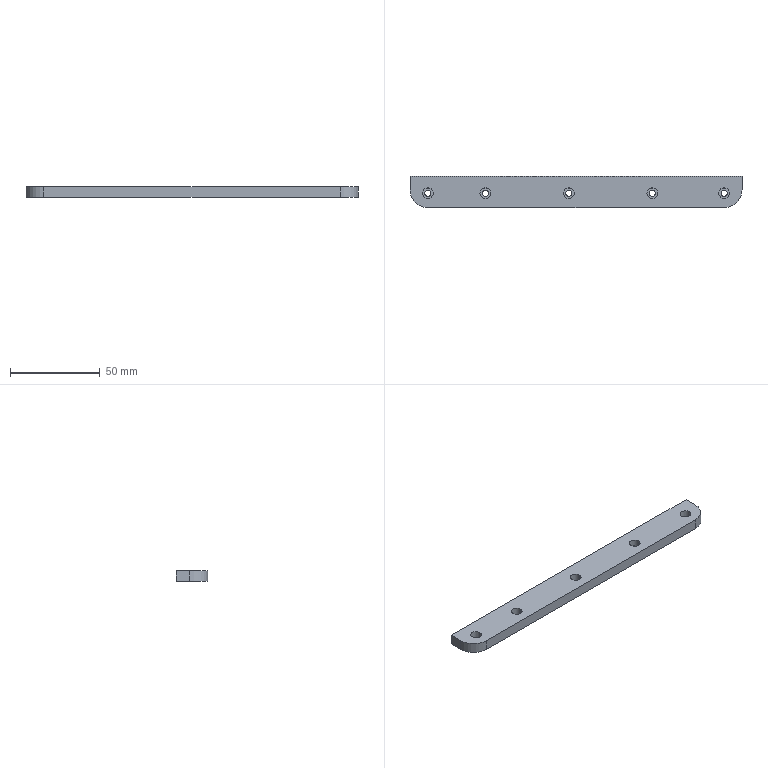Part | STEP file | PN_0009 Default | 1 solid | 33 faces | box 185 x 17.5 x 6 mm | volume 18511 mm3 | cylinder 22 | plane 11 | commonest cylinder face diameters 3.4 x10 6 x10 20 x2
STEP:
#1=CARTESIAN_POINT('',(-85.5,-0.75,2.));
#2=VERTEX_POINT('',#1);
#3=CARTESIAN_POINT('',(-79.5,-0.75,2.));
#4=VERTEX_POINT('',#3);
#5=CARTESIAN_POINT('',(-82.5,-0.75,2.));
#6=DIRECTION('',(0.,0.,1.));
#7=DIRECTION('',(1.,0.,0.));
#8=AXIS2_PLACEMENT_3D('',#5,#6,#7);
#9=CIRCLE('',#8,3.);
#10=EDGE_CURVE('',#2,#4,#9,.T.);
#11=ORIENTED_EDGE('',*,*,#10,.F.);
#12=CARTESIAN_POINT('',(-85.5,-0.75,6.));
#13=VERTEX_POINT('',#12);
#14=CARTESIAN_POINT('',(-85.5,-0.75,6.));
#15=DIRECTION('',(0.,0.,1.));
#16=VECTOR('',#15,1000.);
#17=LINE('',#14,#16);
#18=EDGE_CURVE('',#2,#13,#17,.T.);
#19=ORIENTED_EDGE('',*,*,#18,.T.);
#20=CARTESIAN_POINT('',(-79.5,-0.75,6.));
#21=VERTEX_POINT('',#20);
#22=CARTESIAN_POINT('',(-82.5,-0.75,6.));
#23=DIRECTION('',(0.,0.,1.));
#24=DIRECTION('',(1.,0.,0.));
#25=AXIS2_PLACEMENT_3D('',#22,#23,#24);
#26=CIRCLE('',#25,3.);
#27=EDGE_CURVE('',#13,#21,#26,.T.);
#28=ORIENTED_EDGE('',*,*,#27,.T.);
#29=CARTESIAN_POINT('',(-79.5,-0.75,6.));
#30=DIRECTION('',(0.,0.,1.));
#31=VECTOR('',#30,1000.);
#32=LINE('',#29,#31);
#33=EDGE_CURVE('',#4,#21,#32,.T.);
#34=ORIENTED_EDGE('',*,*,#33,.F.);
#35=EDGE_LOOP('',(#11,#19,#28,#34));
#36=FACE_OUTER_BOUND('',#35,.T.);
#37=CARTESIAN_POINT('',(-82.5,-0.75,6.));
#38=DIRECTION('',(0.,0.,1.));
#39=DIRECTION('',(1.,0.,0.));
#40=AXIS2_PLACEMENT_3D('',#37,#38,#39);
#41=CYLINDRICAL_SURFACE('',#40,3.);
#42=ADVANCED_FACE('',(#36),#41,.F.);
#43=CARTESIAN_POINT('',(-84.2,-0.75,0.));
#44=VERTEX_POINT('',#43);
#45=CARTESIAN_POINT('',(-80.8,-0.75,0.));
#46=VERTEX_POINT('',#45);
#47=CARTESIAN_POINT('',(-82.5,-0.75,0.));
#48=DIRECTION('',(0.,0.,1.));
#49=DIRECTION('',(1.,0.,0.));
#50=AXIS2_PLACEMENT_3D('',#47,#48,#49);
#51=CIRCLE('',#50,1.7);
#52=EDGE_CURVE('',#44,#46,#51,.T.);
#53=ORIENTED_EDGE('',*,*,#52,.F.);
#54=CARTESIAN_POINT('',(-84.2,-0.75,2.));
#55=VERTEX_POINT('',#54);
#56=CARTESIAN_POINT('',(-84.2,-0.75,6.));
#57=DIRECTION('',(0.,0.,1.));
#58=VECTOR('',#57,1000.);
#59=LINE('',#56,#58);
#60=EDGE_CURVE('',#44,#55,#59,.T.);
#61=ORIENTED_EDGE('',*,*,#60,.T.);
#62=CARTESIAN_POINT('',(-80.8,-0.75,2.));
#63=VERTEX_POINT('',#62);
#64=CARTESIAN_POINT('',(-82.5,-0.75,2.));
#65=DIRECTION('',(0.,0.,1.));
#66=DIRECTION('',(1.,0.,0.));
#67=AXIS2_PLACEMENT_3D('',#64,#65,#66);
#68=CIRCLE('',#67,1.7);
#69=EDGE_CURVE('',#55,#63,#68,.T.);
#70=ORIENTED_EDGE('',*,*,#69,.T.);
#71=CARTESIAN_POINT('',(-80.8,-0.75,6.));
#72=DIRECTION('',(0.,0.,1.));
#73=VECTOR('',#72,1000.);
#74=LINE('',#71,#73);
#75=EDGE_CURVE('',#46,#63,#74,.T.);
#76=ORIENTED_EDGE('',*,*,#75,.F.);
#77=EDGE_LOOP('',(#53,#61,#70,#76));
#78=FACE_OUTER_BOUND('',#77,.T.);
#79=CARTESIAN_POINT('',(-82.5,-0.75,6.));
#80=DIRECTION('',(0.,0.,1.));
#81=DIRECTION('',(1.,0.,0.));
#82=AXIS2_PLACEMENT_3D('',#79,#80,#81);
#83=CYLINDRICAL_SURFACE('',#82,1.7);
#84=ADVANCED_FACE('',(#78),#83,.F.);
#85=CARTESIAN_POINT('',(-7.,-0.75,2.));
#86=VERTEX_POINT('',#85);
#87=CARTESIAN_POINT('',(-1.,-0.75,2.));
#88=VERTEX_POINT('',#87);
#89=CARTESIAN_POINT('',(-4.,-0.75,2.));
#90=DIRECTION('',(0.,0.,1.));
#91=DIRECTION('',(1.,0.,0.));
#92=AXIS2_PLACEMENT_3D('',#89,#90,#91);
#93=CIRCLE('',#92,3.);
#94=EDGE_CURVE('',#86,#88,#93,.T.);
#95=ORIENTED_EDGE('',*,*,#94,.F.);
#96=CARTESIAN_POINT('',(-7.,-0.75,6.));
#97=VERTEX_POINT('',#96);
#98=CARTESIAN_POINT('',(-7.,-0.75,6.));
#99=DIRECTION('',(0.,0.,1.));
#100=VECTOR('',#99,1000.);
#101=LINE('',#98,#100);
#102=EDGE_CURVE('',#86,#97,#101,.T.);
#103=ORIENTED_EDGE('',*,*,#102,.T.);
#104=CARTESIAN_POINT('',(-1.,-0.75,6.));
#105=VERTEX_POINT('',#104);
#106=CARTESIAN_POINT('',(-4.,-0.75,6.));
#107=DIRECTION('',(0.,0.,1.));
#108=DIRECTION('',(1.,0.,0.));
#109=AXIS2_PLACEMENT_3D('',#106,#107,#108);
#110=CIRCLE('',#109,3.);
#111=EDGE_CURVE('',#97,#105,#110,.T.);
#112=ORIENTED_EDGE('',*,*,#111,.T.);
#113=CARTESIAN_POINT('',(-1.,-0.75,6.));
#114=DIRECTION('',(0.,0.,1.));
#115=VECTOR('',#114,1000.);
#116=LINE('',#113,#115);
#117=EDGE_CURVE('',#88,#105,#116,.T.);
#118=ORIENTED_EDGE('',*,*,#117,.F.);
#119=EDGE_LOOP('',(#95,#103,#112,#118));
#120=FACE_OUTER_BOUND('',#119,.T.);
#121=CARTESIAN_POINT('',(-4.,-0.75,6.));
#122=DIRECTION('',(0.,0.,1.));
#123=DIRECTION('',(1.,0.,0.));
#124=AXIS2_PLACEMENT_3D('',#121,#122,#123);
#125=CYLINDRICAL_SURFACE('',#124,3.);
#126=ADVANCED_FACE('',(#120),#125,.F.);
#127=CARTESIAN_POINT('',(-5.7,-0.75,0.));
#128=VERTEX_POINT('',#127);
#129=CARTESIAN_POINT('',(-2.3,-0.75,0.));
#130=VERTEX_POINT('',#129);
#131=CARTESIAN_POINT('',(-4.,-0.75,0.));
#132=DIRECTION('',(0.,0.,1.));
#133=DIRECTION('',(1.,0.,0.));
#134=AXIS2_PLACEMENT_3D('',#131,#132,#133);
#135=CIRCLE('',#134,1.7);
#136=EDGE_CURVE('',#128,#130,#135,.T.);
#137=ORIENTED_EDGE('',*,*,#136,.F.);
#138=CARTESIAN_POINT('',(-5.7,-0.75,2.));
#139=VERTEX_POINT('',#138);
#140=CARTESIAN_POINT('',(-5.7,-0.75,6.));
#141=DIRECTION('',(0.,0.,1.));
#142=VECTOR('',#141,1000.);
#143=LINE('',#140,#142);
#144=EDGE_CURVE('',#128,#139,#143,.T.);
#145=ORIENTED_EDGE('',*,*,#144,.T.);
#146=CARTESIAN_POINT('',(-2.3,-0.75,2.));
#147=VERTEX_POINT('',#146);
#148=CARTESIAN_POINT('',(-4.,-0.75,2.));
#149=DIRECTION('',(0.,0.,1.));
#150=DIRECTION('',(1.,0.,0.));
#151=AXIS2_PLACEMENT_3D('',#148,#149,#150);
#152=CIRCLE('',#151,1.7);
#153=EDGE_CURVE('',#139,#147,#152,.T.);
#154=ORIENTED_EDGE('',*,*,#153,.T.);
#155=CARTESIAN_POINT('',(-2.3,-0.75,6.));
#156=DIRECTION('',(0.,0.,1.));
#157=VECTOR('',#156,1000.);
#158=LINE('',#155,#157);
#159=EDGE_CURVE('',#130,#147,#158,.T.);
#160=ORIENTED_EDGE('',*,*,#159,.F.);
#161=EDGE_LOOP('',(#137,#145,#154,#160));
#162=FACE_OUTER_BOUND('',#161,.T.);
#163=CARTESIAN_POINT('',(-4.,-0.75,6.));
#164=DIRECTION('',(0.,0.,1.));
#165=DIRECTION('',(1.,0.,0.));
#166=AXIS2_PLACEMENT_3D('',#163,#164,#165);
#167=CYLINDRICAL_SURFACE('',#166,1.7);
#168=ADVANCED_FACE('',(#162),#167,.F.);
#169=CARTESIAN_POINT('',(39.5,-0.75,2.));
#170=VERTEX_POINT('',#169);
#171=CARTESIAN_POINT('',(45.5,-0.75,2.));
#172=VERTEX_POINT('',#171);
#173=CARTESIAN_POINT('',(42.5,-0.75,2.));
#174=DIRECTION('',(0.,0.,1.));
#175=DIRECTION('',(1.,0.,0.));
#176=AXIS2_PLACEMENT_3D('',#173,#174,#175);
#177=CIRCLE('',#176,3.);
#178=EDGE_CURVE('',#170,#172,#177,.T.);
#179=ORIENTED_EDGE('',*,*,#178,.F.);
#180=CARTESIAN_POINT('',(39.5,-0.75,6.));
#181=VERTEX_POINT('',#180);
#182=CARTESIAN_POINT('',(39.5,-0.75,6.));
#183=DIRECTION('',(0.,0.,1.));
#184=VECTOR('',#183,1000.);
#185=LINE('',#182,#184);
#186=EDGE_CURVE('',#170,#181,#185,.T.);
#187=ORIENTED_EDGE('',*,*,#186,.T.);
#188=CARTESIAN_POINT('',(45.5,-0.75,6.));
#189=VERTEX_POINT('',#188);
#190=CARTESIAN_POINT('',(42.5,-0.75,6.));
#191=DIRECTION('',(0.,0.,1.));
#192=DIRECTION('',(1.,0.,0.));
#193=AXIS2_PLACEMENT_3D('',#190,#191,#192);
#194=CIRCLE('',#193,3.);
#195=EDGE_CURVE('',#181,#189,#194,.T.);
#196=ORIENTED_EDGE('',*,*,#195,.T.);
#197=CARTESIAN_POINT('',(45.5,-0.75,6.));
#198=DIRECTION('',(0.,0.,1.));
#199=VECTOR('',#198,1000.);
#200=LINE('',#197,#199);
#201=EDGE_CURVE('',#172,#189,#200,.T.);
#202=ORIENTED_EDGE('',*,*,#201,.F.);
#203=EDGE_LOOP('',(#179,#187,#196,#202));
#204=FACE_OUTER_BOUND('',#203,.T.);
#205=CARTESIAN_POINT('',(42.5,-0.75,6.));
#206=DIRECTION('',(0.,0.,1.));
#207=DIRECTION('',(1.,0.,0.));
#208=AXIS2_PLACEMENT_3D('',#205,#206,#207);
#209=CYLINDRICAL_SURFACE('',#208,3.);
#210=ADVANCED_FACE('',(#204),#209,.F.);
#211=CARTESIAN_POINT('',(40.8,-0.75,0.));
#212=VERTEX_POINT('',#211);
#213=CARTESIAN_POINT('',(44.2,-0.75,0.));
#214=VERTEX_POINT('',#213);
#215=CARTESIAN_POINT('',(42.5,-0.75,0.));
#216=DIRECTION('',(0.,0.,1.));
#217=DIRECTION('',(1.,0.,0.));
#218=AXIS2_PLACEMENT_3D('',#215,#216,#217);
#219=CIRCLE('',#218,1.7);
#220=EDGE_CURVE('',#212,#214,#219,.T.);
#221=ORIENTED_EDGE('',*,*,#220,.F.);
#222=CARTESIAN_POINT('',(40.8,-0.75,2.));
#223=VERTEX_POINT('',#222);
#224=CARTESIAN_POINT('',(40.8,-0.75,6.));
#225=DIRECTION('',(0.,0.,1.));
#226=VECTOR('',#225,1000.);
#227=LINE('',#224,#226);
#228=EDGE_CURVE('',#212,#223,#227,.T.);
#229=ORIENTED_EDGE('',*,*,#228,.T.);
#230=CARTESIAN_POINT('',(44.2,-0.75,2.));
#231=VERTEX_POINT('',#230);
#232=CARTESIAN_POINT('',(42.5,-0.75,2.));
#233=DIRECTION('',(0.,0.,1.));
#234=DIRECTION('',(1.,0.,0.));
#235=AXIS2_PLACEMENT_3D('',#232,#233,#234);
#236=CIRCLE('',#235,1.7);
#237=EDGE_CURVE('',#223,#231,#236,.T.);
#238=ORIENTED_EDGE('',*,*,#237,.T.);
#239=CARTESIAN_POINT('',(44.2,-0.75,6.));
#240=DIRECTION('',(0.,0.,1.));
#241=VECTOR('',#240,1000.);
#242=LINE('',#239,#241);
#243=EDGE_CURVE('',#214,#231,#242,.T.);
#244=ORIENTED_EDGE('',*,*,#243,.F.);
#245=EDGE_LOOP('',(#221,#229,#238,#244));
#246=FACE_OUTER_BOUND('',#245,.T.);
#247=CARTESIAN_POINT('',(42.5,-0.75,6.));
#248=DIRECTION('',(0.,0.,1.));
#249=DIRECTION('',(1.,0.,0.));
#250=AXIS2_PLACEMENT_3D('',#247,#248,#249);
#251=CYLINDRICAL_SURFACE('',#250,1.7);
#252=ADVANCED_FACE('',(#246),#251,.F.);
#253=CARTESIAN_POINT('',(-53.5,-0.75,2.));
#254=VERTEX_POINT('',#253);
#255=CARTESIAN_POINT('',(-47.5,-0.75,2.));
#256=VERTEX_POINT('',#255);
#257=CARTESIAN_POINT('',(-50.5,-0.75,2.));
#258=DIRECTION('',(0.,0.,1.));
#259=DIRECTION('',(1.,0.,0.));
#260=AXIS2_PLACEMENT_3D('',#257,#258,#259);
#261=CIRCLE('',#260,3.);
#262=EDGE_CURVE('',#254,#256,#261,.T.);
#263=ORIENTED_EDGE('',*,*,#262,.F.);
#264=CARTESIAN_POINT('',(-53.5,-0.75,6.));
#265=VERTEX_POINT('',#264);
#266=CARTESIAN_POINT('',(-53.5,-0.75,6.));
#267=DIRECTION('',(0.,0.,1.));
#268=VECTOR('',#267,1000.);
#269=LINE('',#266,#268);
#270=EDGE_CURVE('',#254,#265,#269,.T.);
#271=ORIENTED_EDGE('',*,*,#270,.T.);
#272=CARTESIAN_POINT('',(-47.5,-0.75,6.));
#273=VERTEX_POINT('',#272);
#274=CARTESIAN_POINT('',(-50.5,-0.75,6.));
#275=DIRECTION('',(0.,0.,1.));
#276=DIRECTION('',(1.,0.,0.));
#277=AXIS2_PLACEMENT_3D('',#274,#275,#276);
#278=CIRCLE('',#277,3.);
#279=EDGE_CURVE('',#265,#273,#278,.T.);
#280=ORIENTED_EDGE('',*,*,#279,.T.);
#281=CARTESIAN_POINT('',(-47.5,-0.75,6.));
#282=DIRECTION('',(0.,0.,1.));
#283=VECTOR('',#282,1000.);
#284=LINE('',#281,#283);
#285=EDGE_CURVE('',#256,#273,#284,.T.);
#286=ORIENTED_EDGE('',*,*,#285,.F.);
#287=EDGE_LOOP('',(#263,#271,#280,#286));
#288=FACE_OUTER_BOUND('',#287,.T.);
#289=CARTESIAN_POINT('',(-50.5,-0.75,6.));
#290=DIRECTION('',(0.,0.,1.));
#291=DIRECTION('',(1.,0.,0.));
#292=AXIS2_PLACEMENT_3D('',#289,#290,#291);
#293=CYLINDRICAL_SURFACE('',#292,3.);
#294=ADVANCED_FACE('',(#288),#293,.F.);
#295=CARTESIAN_POINT('',(-52.2,-0.75,0.));
#296=VERTEX_POINT('',#295);
#297=CARTESIAN_POINT('',(-48.8,-0.75,0.));
#298=VERTEX_POINT('',#297);
#299=CARTESIAN_POINT('',(-50.5,-0.75,0.));
#300=DIRECTION('',(0.,0.,1.));
#301=DIRECTION('',(1.,0.,0.));
#302=AXIS2_PLACEMENT_3D('',#299,#300,#301);
#303=CIRCLE('',#302,1.7);
#304=EDGE_CURVE('',#296,#298,#303,.T.);
#305=ORIENTED_EDGE('',*,*,#304,.F.);
#306=CARTESIAN_POINT('',(-52.2,-0.75,2.));
#307=VERTEX_POINT('',#306);
#308=CARTESIAN_POINT('',(-52.2,-0.75,6.));
#309=DIRECTION('',(0.,0.,1.));
#310=VECTOR('',#309,1000.);
#311=LINE('',#308,#310);
#312=EDGE_CURVE('',#296,#307,#311,.T.);
#313=ORIENTED_EDGE('',*,*,#312,.T.);
#314=CARTESIAN_POINT('',(-48.8,-0.75,2.));
#315=VERTEX_POINT('',#314);
#316=CARTESIAN_POINT('',(-50.5,-0.75,2.));
#317=DIRECTION('',(0.,0.,1.));
#318=DIRECTION('',(1.,0.,0.));
#319=AXIS2_PLACEMENT_3D('',#316,#317,#318);
#320=CIRCLE('',#319,1.7);
#321=EDGE_CURVE('',#307,#315,#320,.T.);
#322=ORIENTED_EDGE('',*,*,#321,.T.);
#323=CARTESIAN_POINT('',(-48.8,-0.75,6.));
#324=DIRECTION('',(0.,0.,1.));
#325=VECTOR('',#324,1000.);
#326=LINE('',#323,#325);
#327=EDGE_CURVE('',#298,#315,#326,.T.);
#328=ORIENTED_EDGE('',*,*,#327,.F.);
#329=EDGE_LOOP('',(#305,#313,#322,#328));
#330=FACE_OUTER_BOUND('',#329,.T.);
#331=CARTESIAN_POINT('',(-50.5,-0.75,6.));
#332=DIRECTION('',(0.,0.,1.));
#333=DIRECTION('',(1.,0.,0.));
#334=AXIS2_PLACEMENT_3D('',#331,#332,#333);
#335=CYLINDRICAL_SURFACE('',#334,1.7);
#336=ADVANCED_FACE('',(#330),#335,.F.);
#337=CARTESIAN_POINT('',(79.5,-0.75,2.));
#338=VERTEX_POINT('',#337);
#339=CARTESIAN_POINT('',(85.5,-0.75,2.));
#340=VERTEX_POINT('',#339);
#341=CARTESIAN_POINT('',(82.5,-0.75,2.));
#342=DIRECTION('',(0.,0.,1.));
#343=DIRECTION('',(1.,0.,0.));
#344=AXIS2_PLACEMENT_3D('',#341,#342,#343);
#345=CIRCLE('',#344,3.);
#346=EDGE_CURVE('',#338,#340,#345,.T.);
#347=ORIENTED_EDGE('',*,*,#346,.F.);
#348=CARTESIAN_POINT('',(79.5,-0.75,6.));
#349=VERTEX_POINT('',#348);
#350=CARTESIAN_POINT('',(79.5,-0.75,6.));
#351=DIRECTION('',(0.,0.,1.));
#352=VECTOR('',#351,1000.);
#353=LINE('',#350,#352);
#354=EDGE_CURVE('',#338,#349,#353,.T.);
#355=ORIENTED_EDGE('',*,*,#354,.T.);
#356=CARTESIAN_POINT('',(85.5,-0.75,6.));
#357=VERTEX_POINT('',#356);
#358=CARTESIAN_POINT('',(82.5,-0.75,6.));
#359=DIRECTION('',(0.,0.,1.));
#360=DIRECTION('',(1.,0.,0.));
#361=AXIS2_PLACEMENT_3D('',#358,#359,#360);
#362=CIRCLE('',#361,3.);
#363=EDGE_CURVE('',#349,#357,#362,.T.);
#364=ORIENTED_EDGE('',*,*,#363,.T.);
#365=CARTESIAN_POINT('',(85.5,-0.75,6.));
#366=DIRECTION('',(0.,0.,1.));
#367=VECTOR('',#366,1000.);
#368=LINE('',#365,#367);
#369=EDGE_CURVE('',#340,#357,#368,.T.);
#370=ORIENTED_EDGE('',*,*,#369,.F.);
#371=EDGE_LOOP('',(#347,#355,#364,#370));
#372=FACE_OUTER_BOUND('',#371,.T.);
#373=CARTESIAN_POINT('',(82.5,-0.75,6.));
#374=DIRECTION('',(0.,0.,1.));
#375=DIRECTION('',(1.,0.,0.));
#376=AXIS2_PLACEMENT_3D('',#373,#374,#375);
#377=CYLINDRICAL_SURFACE('',#376,3.);
#378=ADVANCED_FACE('',(#372),#377,.F.);
#379=CARTESIAN_POINT('',(80.8,-0.75,0.));
#380=VERTEX_POINT('',#379);
#381=CARTESIAN_POINT('',(84.2,-0.75,0.));
#382=VERTEX_POINT('',#381);
#383=CARTESIAN_POINT('',(82.5,-0.75,0.));
#384=DIRECTION('',(0.,0.,1.));
#385=DIRECTION('',(1.,0.,0.));
#386=AXIS2_PLACEMENT_3D('',#383,#384,#385);
#387=CIRCLE('',#386,1.7);
#388=EDGE_CURVE('',#380,#382,#387,.T.);
#389=ORIENTED_EDGE('',*,*,#388,.F.);
#390=CARTESIAN_POINT('',(80.8,-0.75,2.));
#391=VERTEX_POINT('',#390);
#392=CARTESIAN_POINT('',(80.8,-0.75,6.));
#393=DIRECTION('',(0.,0.,1.));
#394=VECTOR('',#393,1000.);
#395=LINE('',#392,#394);
#396=EDGE_CURVE('',#380,#391,#395,.T.);
#397=ORIENTED_EDGE('',*,*,#396,.T.);
#398=CARTESIAN_POINT('',(84.2,-0.75,2.));
#399=VERTEX_POINT('',#398);
#400=CARTESIAN_POINT('',(82.5,-0.75,2.));
#401=DIRECTION('',(0.,0.,1.));
#402=DIRECTION('',(1.,0.,0.));
#403=AXIS2_PLACEMENT_3D('',#400,#401,#402);
#404=CIRCLE('',#403,1.7);
#405=EDGE_CURVE('',#391,#399,#404,.T.);
#406=ORIENTED_EDGE('',*,*,#405,.T.);
#407=CARTESIAN_POINT('',(84.2,-0.75,6.));
#408=DIRECTION('',(0.,0.,1.));
#409=VECTOR('',#408,1000.);
#410=LINE('',#407,#409);
#411=EDGE_CURVE('',#382,#399,#410,.T.);
#412=ORIENTED_EDGE('',*,*,#411,.F.);
#413=EDGE_LOOP('',(#389,#397,#406,#412));
#414=FACE_OUTER_BOUND('',#413,.T.);
#415=CARTESIAN_POINT('',(82.5,-0.75,6.));
#416=DIRECTION('',(0.,0.,1.));
#417=DIRECTION('',(1.,0.,0.));
#418=AXIS2_PLACEMENT_3D('',#415,#416,#417);
#419=CYLINDRICAL_SURFACE('',#418,1.7);
#420=ADVANCED_FACE('',(#414),#419,.F.);
#421=CARTESIAN_POINT('',(92.5,1.25,6.));
#422=VERTEX_POINT('',#421);
#423=CARTESIAN_POINT('',(92.5,8.75,6.));
#424=VERTEX_POINT('',#423);
#425=CARTESIAN_POINT('',(92.5,8.75,6.));
#426=DIRECTION('',(0.,1.,0.));
#427=VECTOR('',#426,1000.);
#428=LINE('',#425,#427);
#429=EDGE_CURVE('',#422,#424,#428,.T.);
#430=ORIENTED_EDGE('',*,*,#429,.F.);
#431=CARTESIAN_POINT('',(92.5,1.25,0.));
#432=VERTEX_POINT('',#431);
#433=CARTESIAN_POINT('',(92.5,1.25,6.));
#434=DIRECTION('',(0.,0.,-1.));
#435=VECTOR('',#434,1000.);
#436=LINE('',#433,#435);
#437=EDGE_CURVE('',#422,#432,#436,.T.);
#438=ORIENTED_EDGE('',*,*,#437,.T.);
#439=CARTESIAN_POINT('',(92.5,8.75,0.));
#440=VERTEX_POINT('',#439);
#441=CARTESIAN_POINT('',(92.5,8.75,0.));
#442=DIRECTION('',(0.,1.,0.));
#443=VECTOR('',#442,1000.);
#444=LINE('',#441,#443);
#445=EDGE_CURVE('',#432,#440,#444,.T.);
#446=ORIENTED_EDGE('',*,*,#445,.T.);
#447=CARTESIAN_POINT('',(92.5,8.75,6.));
#448=DIRECTION('',(0.,0.,-1.));
#449=VECTOR('',#448,1000.);
#450=LINE('',#447,#449);
#451=EDGE_CURVE('',#424,#440,#450,.T.);
#452=ORIENTED_EDGE('',*,*,#451,.F.);
#453=EDGE_LOOP('',(#430,#438,#446,#452));
#454=FACE_OUTER_BOUND('',#453,.T.);
#455=CARTESIAN_POINT('',(92.5,8.75,6.));
#456=DIRECTION('',(-1.,0.,0.));
#457=DIRECTION('',(0.,0.,1.));
#458=AXIS2_PLACEMENT_3D('',#455,#456,#457);
#459=PLANE('',#458);
#460=ADVANCED_FACE('',(#454),#459,.F.);
#461=CARTESIAN_POINT('',(-92.5,8.75,0.));
#462=VERTEX_POINT('',#461);
#463=CARTESIAN_POINT('',(-92.5,8.75,0.));
#464=DIRECTION('',(-1.,0.,0.));
#465=VECTOR('',#464,1000.);
#466=LINE('',#463,#465);
#467=EDGE_CURVE('',#440,#462,#466,.T.);
#468=ORIENTED_EDGE('',*,*,#467,.T.);
#469=CARTESIAN_POINT('',(-92.5,8.75,6.));
#470=VERTEX_POINT('',#469);
#471=CARTESIAN_POINT('',(-92.5,8.75,6.));
#472=DIRECTION('',(0.,0.,-1.));
#473=VECTOR('',#472,1000.);
#474=LINE('',#471,#473);
#475=EDGE_CURVE('',#470,#462,#474,.T.);
#476=ORIENTED_EDGE('',*,*,#475,.F.);
#477=CARTESIAN_POINT('',(-92.5,8.75,6.));
#478=DIRECTION('',(-1.,0.,0.));
#479=VECTOR('',#478,1000.);
#480=LINE('',#477,#479);
#481=EDGE_CURVE('',#424,#470,#480,.T.);
#482=ORIENTED_EDGE('',*,*,#481,.F.);
#483=ORIENTED_EDGE('',*,*,#451,.T.);
#484=EDGE_LOOP('',(#468,#476,#482,#483));
#485=FACE_OUTER_BOUND('',#484,.T.);
#486=CARTESIAN_POINT('',(-92.5,8.75,6.));
#487=DIRECTION('',(0.,-1.,0.));
#488=DIRECTION('',(0.,0.,-1.));
#489=AXIS2_PLACEMENT_3D('',#486,#487,#488);
#490=PLANE('',#489);
#491=ADVANCED_FACE('',(#485),#490,.F.);
#492=CARTESIAN_POINT('',(-92.5,1.25,0.));
#493=VERTEX_POINT('',#492);
#494=CARTESIAN_POINT('',(-92.5,8.75,0.));
#495=DIRECTION('',(0.,-1.,0.));
#496=VECTOR('',#495,1000.);
#497=LINE('',#494,#496);
#498=EDGE_CURVE('',#462,#493,#497,.T.);
#499=ORIENTED_EDGE('',*,*,#498,.T.);
#500=CARTESIAN_POINT('',(-92.5,1.25,6.));
#501=VERTEX_POINT('',#500);
#502=CARTESIAN_POINT('',(-92.5,1.25,6.));
#503=DIRECTION('',(0.,0.,1.));
#504=VECTOR('',#503,1000.);
#505=LINE('',#502,#504);
#506=EDGE_CURVE('',#493,#501,#505,.T.);
#507=ORIENTED_EDGE('',*,*,#506,.T.);
#508=CARTESIAN_POINT('',(-92.5,8.75,6.));
#509=DIRECTION('',(0.,-1.,0.));
#510=VECTOR('',#509,1000.);
#511=LINE('',#508,#510);
#512=EDGE_CURVE('',#470,#501,#511,.T.);
#513=ORIENTED_EDGE('',*,*,#512,.F.);
#514=ORIENTED_EDGE('',*,*,#475,.T.);
#515=EDGE_LOOP('',(#499,#507,#513,#514));
#516=FACE_OUTER_BOUND('',#515,.T.);
#517=CARTESIAN_POINT('',(-92.5,8.75,6.));
#518=DIRECTION('',(1.,0.,0.));
#519=DIRECTION('',(0.,0.,-1.));
#520=AXIS2_PLACEMENT_3D('',#517,#518,#519);
#521=PLANE('',#520);
#522=ADVANCED_FACE('',(#516),#521,.F.);
#523=CARTESIAN_POINT('',(-82.5,-8.75,0.));
#524=VERTEX_POINT('',#523);
#525=CARTESIAN_POINT('',(82.5,-8.75,0.));
#526=VERTEX_POINT('',#525);
#527=CARTESIAN_POINT('',(-92.5,-8.75,0.));
#528=DIRECTION('',(1.,0.,0.));
#529=VECTOR('',#528,1000.);
#530=LINE('',#527,#529);
#531=EDGE_CURVE('',#524,#526,#530,.T.);
#532=ORIENTED_EDGE('',*,*,#531,.T.);
#533=CARTESIAN_POINT('',(82.5,-8.75,6.));
#534=VERTEX_POINT('',#533);
#535=CARTESIAN_POINT('',(82.5,-8.75,6.));
#536=DIRECTION('',(0.,0.,1.));
#537=VECTOR('',#536,1000.);
#538=LINE('',#535,#537);
#539=EDGE_CURVE('',#526,#534,#538,.T.);
#540=ORIENTED_EDGE('',*,*,#539,.T.);
#541=CARTESIAN_POINT('',(-82.5,-8.75,6.));
#542=VERTEX_POINT('',#541);
#543=CARTESIAN_POINT('',(-92.5,-8.75,6.));
#544=DIRECTION('',(1.,0.,0.));
#545=VECTOR('',#544,1000.);
#546=LINE('',#543,#545);
#547=EDGE_CURVE('',#542,#534,#546,.T.);
#548=ORIENTED_EDGE('',*,*,#547,.F.);
#549=CARTESIAN_POINT('',(-82.5,-8.75,6.));
#550=DIRECTION('',(0.,0.,-1.));
#551=VECTOR('',#550,1000.);
#552=LINE('',#549,#551);
#553=EDGE_CURVE('',#542,#524,#552,.T.);
#554=ORIENTED_EDGE('',*,*,#553,.T.);
#555=EDGE_LOOP('',(#532,#540,#548,#554));
#556=FACE_OUTER_BOUND('',#555,.T.);
#557=CARTESIAN_POINT('',(-92.5,-8.75,6.));
#558=DIRECTION('',(0.,1.,0.));
#559=DIRECTION('',(0.,0.,1.));
#560=AXIS2_PLACEMENT_3D('',#557,#558,#559);
#561=PLANE('',#560);
#562=ADVANCED_FACE('',(#556),#561,.F.);
#563=CARTESIAN_POINT('',(-82.5,-0.75,6.));
#564=DIRECTION('',(0.,0.,1.));
#565=DIRECTION('',(1.,0.,0.));
#566=AXIS2_PLACEMENT_3D('',#563,#564,#565);
#567=CIRCLE('',#566,3.);
#568=EDGE_CURVE('',#21,#13,#567,.T.);
#569=ORIENTED_EDGE('',*,*,#568,.F.);
#570=ORIENTED_EDGE('',*,*,#27,.F.);
#571=EDGE_LOOP('',(#569,#570));
#572=FACE_BOUND('',#571,.T.);
#573=CARTESIAN_POINT('',(-4.,-0.75,6.));
#574=DIRECTION('',(0.,0.,1.));
#575=DIRECTION('',(1.,0.,0.));
#576=AXIS2_PLACEMENT_3D('',#573,#574,#575);
#577=CIRCLE('',#576,3.);
#578=EDGE_CURVE('',#105,#97,#577,.T.);
#579=ORIENTED_EDGE('',*,*,#578,.F.);
#580=ORIENTED_EDGE('',*,*,#111,.F.);
#581=EDGE_LOOP('',(#579,#580));
#582=FACE_BOUND('',#581,.T.);
#583=CARTESIAN_POINT('',(42.5,-0.75,6.));
#584=DIRECTION('',(0.,0.,1.));
#585=DIRECTION('',(1.,0.,0.));
#586=AXIS2_PLACEMENT_3D('',#583,#584,#585);
#587=CIRCLE('',#586,3.);
#588=EDGE_CURVE('',#189,#181,#587,.T.);
#589=ORIENTED_EDGE('',*,*,#588,.F.);
#590=ORIENTED_EDGE('',*,*,#195,.F.);
#591=EDGE_LOOP('',(#589,#590));
#592=FACE_BOUND('',#591,.T.);
#593=CARTESIAN_POINT('',(-50.5,-0.75,6.));
#594=DIRECTION('',(0.,0.,1.));
#595=DIRECTION('',(1.,0.,0.));
#596=AXIS2_PLACEMENT_3D('',#593,#594,#595);
#597=CIRCLE('',#596,3.);
#598=EDGE_CURVE('',#273,#265,#597,.T.);
#599=ORIENTED_EDGE('',*,*,#598,.F.);
#600=ORIENTED_EDGE('',*,*,#279,.F.);
#601=EDGE_LOOP('',(#599,#600));
#602=FACE_BOUND('',#601,.T.);
#603=CARTESIAN_POINT('',(82.5,-0.75,6.));
#604=DIRECTION('',(0.,0.,1.));
#605=DIRECTION('',(1.,0.,0.));
#606=AXIS2_PLACEMENT_3D('',#603,#604,#605);
#607=CIRCLE('',#606,3.);
#608=EDGE_CURVE('',#357,#349,#607,.T.);
#609=ORIENTED_EDGE('',*,*,#608,.F.);
#610=ORIENTED_EDGE('',*,*,#363,.F.);
#611=EDGE_LOOP('',(#609,#610));
#612=FACE_BOUND('',#611,.T.);
#613=ORIENTED_EDGE('',*,*,#547,.T.);
#614=CARTESIAN_POINT('',(82.5,1.25,6.));
#615=DIRECTION('',(0.,0.,1.));
#616=DIRECTION('',(1.,0.,0.));
#617=AXIS2_PLACEMENT_3D('',#614,#615,#616);
#618=CIRCLE('',#617,10.);
#619=EDGE_CURVE('',#534,#422,#618,.T.);
#620=ORIENTED_EDGE('',*,*,#619,.T.);
#621=ORIENTED_EDGE('',*,*,#429,.T.);
#622=ORIENTED_EDGE('',*,*,#481,.T.);
#623=ORIENTED_EDGE('',*,*,#512,.T.);
#624=CARTESIAN_POINT('',(-82.5,1.25,6.));
#625=DIRECTION('',(0.,0.,1.));
#626=DIRECTION('',(1.,0.,0.));
#627=AXIS2_PLACEMENT_3D('',#624,#625,#626);
#628=CIRCLE('',#627,10.);
#629=EDGE_CURVE('',#501,#542,#628,.T.);
#630=ORIENTED_EDGE('',*,*,#629,.T.);
#631=EDGE_LOOP('',(#613,#620,#621,#622,#623,#630));
#632=FACE_OUTER_BOUND('',#631,.T.);
#633=CARTESIAN_POINT('',(0.,0.,6.));
#634=DIRECTION('',(0.,0.,1.));
#635=DIRECTION('',(1.,0.,0.));
#636=AXIS2_PLACEMENT_3D('',#633,#634,#635);
#637=PLANE('',#636);
#638=ADVANCED_FACE('',(#572,#582,#592,#602,#612,#632),#637,.T.);
#639=CARTESIAN_POINT('',(-82.5,-0.75,0.));
#640=DIRECTION('',(0.,0.,1.));
#641=DIRECTION('',(1.,0.,0.));
#642=AXIS2_PLACEMENT_3D('',#639,#640,#641);
#643=CIRCLE('',#642,1.7);
#644=EDGE_CURVE('',#46,#44,#643,.T.);
#645=ORIENTED_EDGE('',*,*,#644,.T.);
#646=ORIENTED_EDGE('',*,*,#52,.T.);
#647=EDGE_LOOP('',(#645,#646));
#648=FACE_BOUND('',#647,.T.);
#649=CARTESIAN_POINT('',(-4.,-0.75,0.));
#650=DIRECTION('',(0.,0.,1.));
#651=DIRECTION('',(1.,0.,0.));
#652=AXIS2_PLACEMENT_3D('',#649,#650,#651);
#653=CIRCLE('',#652,1.7);
#654=EDGE_CURVE('',#130,#128,#653,.T.);
#655=ORIENTED_EDGE('',*,*,#654,.T.);
#656=ORIENTED_EDGE('',*,*,#136,.T.);
#657=EDGE_LOOP('',(#655,#656));
#658=FACE_BOUND('',#657,.T.);
#659=CARTESIAN_POINT('',(42.5,-0.75,0.));
#660=DIRECTION('',(0.,0.,1.));
#661=DIRECTION('',(1.,0.,0.));
#662=AXIS2_PLACEMENT_3D('',#659,#660,#661);
#663=CIRCLE('',#662,1.7);
#664=EDGE_CURVE('',#214,#212,#663,.T.);
#665=ORIENTED_EDGE('',*,*,#664,.T.);
#666=ORIENTED_EDGE('',*,*,#220,.T.);
#667=EDGE_LOOP('',(#665,#666));
#668=FACE_BOUND('',#667,.T.);
#669=CARTESIAN_POINT('',(-50.5,-0.75,0.));
#670=DIRECTION('',(0.,0.,1.));
#671=DIRECTION('',(1.,0.,0.));
#672=AXIS2_PLACEMENT_3D('',#669,#670,#671);
#673=CIRCLE('',#672,1.7);
#674=EDGE_CURVE('',#298,#296,#673,.T.);
#675=ORIENTED_EDGE('',*,*,#674,.T.);
#676=ORIENTED_EDGE('',*,*,#304,.T.);
#677=EDGE_LOOP('',(#675,#676));
#678=FACE_BOUND('',#677,.T.);
#679=CARTESIAN_POINT('',(82.5,-0.75,0.));
#680=DIRECTION('',(0.,0.,1.));
#681=DIRECTION('',(1.,0.,0.));
#682=AXIS2_PLACEMENT_3D('',#679,#680,#681);
#683=CIRCLE('',#682,1.7);
#684=EDGE_CURVE('',#382,#380,#683,.T.);
#685=ORIENTED_EDGE('',*,*,#684,.T.);
#686=ORIENTED_EDGE('',*,*,#388,.T.);
#687=EDGE_LOOP('',(#685,#686));
#688=FACE_BOUND('',#687,.T.);
#689=ORIENTED_EDGE('',*,*,#445,.F.);
#690=CARTESIAN_POINT('',(82.5,1.25,0.));
#691=DIRECTION('',(0.,0.,-1.));
#692=DIRECTION('',(1.,0.,0.));
#693=AXIS2_PLACEMENT_3D('',#690,#691,#692);
#694=CIRCLE('',#693,10.);
#695=EDGE_CURVE('',#432,#526,#694,.T.);
#696=ORIENTED_EDGE('',*,*,#695,.T.);
#697=ORIENTED_EDGE('',*,*,#531,.F.);
#698=CARTESIAN_POINT('',(-82.5,1.25,0.));
#699=DIRECTION('',(0.,0.,-1.));
#700=DIRECTION('',(1.,0.,0.));
#701=AXIS2_PLACEMENT_3D('',#698,#699,#700);
#702=CIRCLE('',#701,10.);
#703=EDGE_CURVE('',#524,#493,#702,.T.);
#704=ORIENTED_EDGE('',*,*,#703,.T.);
#705=ORIENTED_EDGE('',*,*,#498,.F.);
#706=ORIENTED_EDGE('',*,*,#467,.F.);
#707=EDGE_LOOP('',(#689,#696,#697,#704,#705,#706));
#708=FACE_OUTER_BOUND('',#707,.T.);
#709=CARTESIAN_POINT('',(0.,0.,0.));
#710=DIRECTION('',(0.,0.,1.));
#711=DIRECTION('',(1.,0.,0.));
#712=AXIS2_PLACEMENT_3D('',#709,#710,#711);
#713=PLANE('',#712);
#714=ADVANCED_FACE('',(#648,#658,#668,#678,#688,#708),#713,.F.);
#715=ORIENTED_EDGE('',*,*,#396,.F.);
#716=ORIENTED_EDGE('',*,*,#684,.F.);
#717=ORIENTED_EDGE('',*,*,#411,.T.);
#718=CARTESIAN_POINT('',(82.5,-0.75,2.));
#719=DIRECTION('',(0.,0.,1.));
#720=DIRECTION('',(1.,0.,0.));
#721=AXIS2_PLACEMENT_3D('',#718,#719,#720);
#722=CIRCLE('',#721,1.7);
#723=EDGE_CURVE('',#399,#391,#722,.T.);
#724=ORIENTED_EDGE('',*,*,#723,.T.);
#725=EDGE_LOOP('',(#715,#716,#717,#724));
#726=FACE_OUTER_BOUND('',#725,.T.);
#727=CARTESIAN_POINT('',(82.5,-0.75,6.));
#728=DIRECTION('',(0.,0.,1.));
#729=DIRECTION('',(1.,0.,0.));
#730=AXIS2_PLACEMENT_3D('',#727,#728,#729);
#731=CYLINDRICAL_SURFACE('',#730,1.7);
#732=ADVANCED_FACE('',(#726),#731,.F.);
#733=ORIENTED_EDGE('',*,*,#723,.F.);
#734=ORIENTED_EDGE('',*,*,#405,.F.);
#735=EDGE_LOOP('',(#733,#734));
#736=FACE_BOUND('',#735,.T.);
#737=CARTESIAN_POINT('',(82.5,-0.75,2.));
#738=DIRECTION('',(0.,0.,1.));
#739=DIRECTION('',(1.,0.,0.));
#740=AXIS2_PLACEMENT_3D('',#737,#738,#739);
#741=CIRCLE('',#740,3.);
#742=EDGE_CURVE('',#340,#338,#741,.T.);
#743=ORIENTED_EDGE('',*,*,#742,.T.);
#744=ORIENTED_EDGE('',*,*,#346,.T.);
#745=EDGE_LOOP('',(#743,#744));
#746=FACE_OUTER_BOUND('',#745,.T.);
#747=CARTESIAN_POINT('',(84.2,-0.75,2.));
#748=DIRECTION('',(0.,0.,-1.));
#749=DIRECTION('',(-1.,0.,0.));
#750=AXIS2_PLACEMENT_3D('',#747,#748,#749);
#751=PLANE('',#750);
#752=ADVANCED_FACE('',(#736,#746),#751,.F.);
#753=ORIENTED_EDGE('',*,*,#354,.F.);
#754=ORIENTED_EDGE('',*,*,#742,.F.);
#755=ORIENTED_EDGE('',*,*,#369,.T.);
#756=ORIENTED_EDGE('',*,*,#608,.T.);
#757=EDGE_LOOP('',(#753,#754,#755,#756));
#758=FACE_OUTER_BOUND('',#757,.T.);
#759=CARTESIAN_POINT('',(82.5,-0.75,6.));
#760=DIRECTION('',(0.,0.,1.));
#761=DIRECTION('',(1.,0.,0.));
#762=AXIS2_PLACEMENT_3D('',#759,#760,#761);
#763=CYLINDRICAL_SURFACE('',#762,3.);
#764=ADVANCED_FACE('',(#758),#763,.F.);
#765=ORIENTED_EDGE('',*,*,#312,.F.);
#766=ORIENTED_EDGE('',*,*,#674,.F.);
#767=ORIENTED_EDGE('',*,*,#327,.T.);
#768=CARTESIAN_POINT('',(-50.5,-0.75,2.));
#769=DIRECTION('',(0.,0.,1.));
#770=DIRECTION('',(1.,0.,0.));
#771=AXIS2_PLACEMENT_3D('',#768,#769,#770);
#772=CIRCLE('',#771,1.7);
#773=EDGE_CURVE('',#315,#307,#772,.T.);
#774=ORIENTED_EDGE('',*,*,#773,.T.);
#775=EDGE_LOOP('',(#765,#766,#767,#774));
#776=FACE_OUTER_BOUND('',#775,.T.);
#777=CARTESIAN_POINT('',(-50.5,-0.75,6.));
#778=DIRECTION('',(0.,0.,1.));
#779=DIRECTION('',(1.,0.,0.));
#780=AXIS2_PLACEMENT_3D('',#777,#778,#779);
#781=CYLINDRICAL_SURFACE('',#780,1.7);
#782=ADVANCED_FACE('',(#776),#781,.F.);
#783=ORIENTED_EDGE('',*,*,#773,.F.);
#784=ORIENTED_EDGE('',*,*,#321,.F.);
#785=EDGE_LOOP('',(#783,#784));
#786=FACE_BOUND('',#785,.T.);
#787=CARTESIAN_POINT('',(-50.5,-0.75,2.));
#788=DIRECTION('',(0.,0.,1.));
#789=DIRECTION('',(1.,0.,0.));
#790=AXIS2_PLACEMENT_3D('',#787,#788,#789);
#791=CIRCLE('',#790,3.);
#792=EDGE_CURVE('',#256,#254,#791,.T.);
#793=ORIENTED_EDGE('',*,*,#792,.T.);
#794=ORIENTED_EDGE('',*,*,#262,.T.);
#795=EDGE_LOOP('',(#793,#794));
#796=FACE_OUTER_BOUND('',#795,.T.);
#797=CARTESIAN_POINT('',(-48.8,-0.75,2.));
#798=DIRECTION('',(0.,0.,-1.));
#799=DIRECTION('',(-1.,0.,0.));
#800=AXIS2_PLACEMENT_3D('',#797,#798,#799);
#801=PLANE('',#800);
#802=ADVANCED_FACE('',(#786,#796),#801,.F.);
#803=ORIENTED_EDGE('',*,*,#270,.F.);
#804=ORIENTED_EDGE('',*,*,#792,.F.);
#805=ORIENTED_EDGE('',*,*,#285,.T.);
#806=ORIENTED_EDGE('',*,*,#598,.T.);
#807=EDGE_LOOP('',(#803,#804,#805,#806));
#808=FACE_OUTER_BOUND('',#807,.T.);
#809=CARTESIAN_POINT('',(-50.5,-0.75,6.));
#810=DIRECTION('',(0.,0.,1.));
#811=DIRECTION('',(1.,0.,0.));
#812=AXIS2_PLACEMENT_3D('',#809,#810,#811);
#813=CYLINDRICAL_SURFACE('',#812,3.);
#814=ADVANCED_FACE('',(#808),#813,.F.);
#815=ORIENTED_EDGE('',*,*,#228,.F.);
#816=ORIENTED_EDGE('',*,*,#664,.F.);
#817=ORIENTED_EDGE('',*,*,#243,.T.);
#818=CARTESIAN_POINT('',(42.5,-0.75,2.));
#819=DIRECTION('',(0.,0.,1.));
#820=DIRECTION('',(1.,0.,0.));
#821=AXIS2_PLACEMENT_3D('',#818,#819,#820);
#822=CIRCLE('',#821,1.7);
#823=EDGE_CURVE('',#231,#223,#822,.T.);
#824=ORIENTED_EDGE('',*,*,#823,.T.);
#825=EDGE_LOOP('',(#815,#816,#817,#824));
#826=FACE_OUTER_BOUND('',#825,.T.);
#827=CARTESIAN_POINT('',(42.5,-0.75,6.));
#828=DIRECTION('',(0.,0.,1.));
#829=DIRECTION('',(1.,0.,0.));
#830=AXIS2_PLACEMENT_3D('',#827,#828,#829);
#831=CYLINDRICAL_SURFACE('',#830,1.7);
#832=ADVANCED_FACE('',(#826),#831,.F.);
#833=ORIENTED_EDGE('',*,*,#823,.F.);
#834=ORIENTED_EDGE('',*,*,#237,.F.);
#835=EDGE_LOOP('',(#833,#834));
#836=FACE_BOUND('',#835,.T.);
#837=CARTESIAN_POINT('',(42.5,-0.75,2.));
#838=DIRECTION('',(0.,0.,1.));
#839=DIRECTION('',(1.,0.,0.));
#840=AXIS2_PLACEMENT_3D('',#837,#838,#839);
#841=CIRCLE('',#840,3.);
#842=EDGE_CURVE('',#172,#170,#841,.T.);
#843=ORIENTED_EDGE('',*,*,#842,.T.);
#844=ORIENTED_EDGE('',*,*,#178,.T.);
#845=EDGE_LOOP('',(#843,#844));
#846=FACE_OUTER_BOUND('',#845,.T.);
#847=CARTESIAN_POINT('',(44.2,-0.75,2.));
#848=DIRECTION('',(0.,0.,-1.));
#849=DIRECTION('',(-1.,0.,0.));
#850=AXIS2_PLACEMENT_3D('',#847,#848,#849);
#851=PLANE('',#850);
#852=ADVANCED_FACE('',(#836,#846),#851,.F.);
#853=ORIENTED_EDGE('',*,*,#186,.F.);
#854=ORIENTED_EDGE('',*,*,#842,.F.);
#855=ORIENTED_EDGE('',*,*,#201,.T.);
#856=ORIENTED_EDGE('',*,*,#588,.T.);
#857=EDGE_LOOP('',(#853,#854,#855,#856));
#858=FACE_OUTER_BOUND('',#857,.T.);
#859=CARTESIAN_POINT('',(42.5,-0.75,6.));
#860=DIRECTION('',(0.,0.,1.));
#861=DIRECTION('',(1.,0.,0.));
#862=AXIS2_PLACEMENT_3D('',#859,#860,#861);
#863=CYLINDRICAL_SURFACE('',#862,3.);
#864=ADVANCED_FACE('',(#858),#863,.F.);
#865=ORIENTED_EDGE('',*,*,#144,.F.);
#866=ORIENTED_EDGE('',*,*,#654,.F.);
#867=ORIENTED_EDGE('',*,*,#159,.T.);
#868=CARTESIAN_POINT('',(-4.,-0.75,2.));
#869=DIRECTION('',(0.,0.,1.));
#870=DIRECTION('',(1.,0.,0.));
#871=AXIS2_PLACEMENT_3D('',#868,#869,#870);
#872=CIRCLE('',#871,1.7);
#873=EDGE_CURVE('',#147,#139,#872,.T.);
#874=ORIENTED_EDGE('',*,*,#873,.T.);
#875=EDGE_LOOP('',(#865,#866,#867,#874));
#876=FACE_OUTER_BOUND('',#875,.T.);
#877=CARTESIAN_POINT('',(-4.,-0.75,6.));
#878=DIRECTION('',(0.,0.,1.));
#879=DIRECTION('',(1.,0.,0.));
#880=AXIS2_PLACEMENT_3D('',#877,#878,#879);
#881=CYLINDRICAL_SURFACE('',#880,1.7);
#882=ADVANCED_FACE('',(#876),#881,.F.);
#883=ORIENTED_EDGE('',*,*,#873,.F.);
#884=ORIENTED_EDGE('',*,*,#153,.F.);
#885=EDGE_LOOP('',(#883,#884));
#886=FACE_BOUND('',#885,.T.);
#887=CARTESIAN_POINT('',(-4.,-0.75,2.));
#888=DIRECTION('',(0.,0.,1.));
#889=DIRECTION('',(1.,0.,0.));
#890=AXIS2_PLACEMENT_3D('',#887,#888,#889);
#891=CIRCLE('',#890,3.);
#892=EDGE_CURVE('',#88,#86,#891,.T.);
#893=ORIENTED_EDGE('',*,*,#892,.T.);
#894=ORIENTED_EDGE('',*,*,#94,.T.);
#895=EDGE_LOOP('',(#893,#894));
#896=FACE_OUTER_BOUND('',#895,.T.);
#897=CARTESIAN_POINT('',(-2.3,-0.75,2.));
#898=DIRECTION('',(0.,0.,-1.));
#899=DIRECTION('',(-1.,0.,0.));
#900=AXIS2_PLACEMENT_3D('',#897,#898,#899);
#901=PLANE('',#900);
#902=ADVANCED_FACE('',(#886,#896),#901,.F.);
#903=ORIENTED_EDGE('',*,*,#102,.F.);
#904=ORIENTED_EDGE('',*,*,#892,.F.);
#905=ORIENTED_EDGE('',*,*,#117,.T.);
#906=ORIENTED_EDGE('',*,*,#578,.T.);
#907=EDGE_LOOP('',(#903,#904,#905,#906));
#908=FACE_OUTER_BOUND('',#907,.T.);
#909=CARTESIAN_POINT('',(-4.,-0.75,6.));
#910=DIRECTION('',(0.,0.,1.));
#911=DIRECTION('',(1.,0.,0.));
#912=AXIS2_PLACEMENT_3D('',#909,#910,#911);
#913=CYLINDRICAL_SURFACE('',#912,3.);
#914=ADVANCED_FACE('',(#908),#913,.F.);
#915=ORIENTED_EDGE('',*,*,#60,.F.);
#916=ORIENTED_EDGE('',*,*,#644,.F.);
#917=ORIENTED_EDGE('',*,*,#75,.T.);
#918=CARTESIAN_POINT('',(-82.5,-0.75,2.));
#919=DIRECTION('',(0.,0.,1.));
#920=DIRECTION('',(1.,0.,0.));
#921=AXIS2_PLACEMENT_3D('',#918,#919,#920);
#922=CIRCLE('',#921,1.7);
#923=EDGE_CURVE('',#63,#55,#922,.T.);
#924=ORIENTED_EDGE('',*,*,#923,.T.);
#925=EDGE_LOOP('',(#915,#916,#917,#924));
#926=FACE_OUTER_BOUND('',#925,.T.);
#927=CARTESIAN_POINT('',(-82.5,-0.75,6.));
#928=DIRECTION('',(0.,0.,1.));
#929=DIRECTION('',(1.,0.,0.));
#930=AXIS2_PLACEMENT_3D('',#927,#928,#929);
#931=CYLINDRICAL_SURFACE('',#930,1.7);
#932=ADVANCED_FACE('',(#926),#931,.F.);
#933=ORIENTED_EDGE('',*,*,#923,.F.);
#934=ORIENTED_EDGE('',*,*,#69,.F.);
#935=EDGE_LOOP('',(#933,#934));
#936=FACE_BOUND('',#935,.T.);
#937=CARTESIAN_POINT('',(-82.5,-0.75,2.));
#938=DIRECTION('',(0.,0.,1.));
#939=DIRECTION('',(1.,0.,0.));
#940=AXIS2_PLACEMENT_3D('',#937,#938,#939);
#941=CIRCLE('',#940,3.);
#942=EDGE_CURVE('',#4,#2,#941,.T.);
#943=ORIENTED_EDGE('',*,*,#942,.T.);
#944=ORIENTED_EDGE('',*,*,#10,.T.);
#945=EDGE_LOOP('',(#943,#944));
#946=FACE_OUTER_BOUND('',#945,.T.);
#947=CARTESIAN_POINT('',(-80.8,-0.75,2.));
#948=DIRECTION('',(0.,0.,-1.));
#949=DIRECTION('',(-1.,0.,0.));
#950=AXIS2_PLACEMENT_3D('',#947,#948,#949);
#951=PLANE('',#950);
#952=ADVANCED_FACE('',(#936,#946),#951,.F.);
#953=ORIENTED_EDGE('',*,*,#18,.F.);
#954=ORIENTED_EDGE('',*,*,#942,.F.);
#955=ORIENTED_EDGE('',*,*,#33,.T.);
#956=ORIENTED_EDGE('',*,*,#568,.T.);
#957=EDGE_LOOP('',(#953,#954,#955,#956));
#958=FACE_OUTER_BOUND('',#957,.T.);
#959=CARTESIAN_POINT('',(-82.5,-0.75,6.));
#960=DIRECTION('',(0.,0.,1.));
#961=DIRECTION('',(1.,0.,0.));
#962=AXIS2_PLACEMENT_3D('',#959,#960,#961);
#963=CYLINDRICAL_SURFACE('',#962,3.);
#964=ADVANCED_FACE('',(#958),#963,.F.);
#965=ORIENTED_EDGE('',*,*,#619,.F.);
#966=ORIENTED_EDGE('',*,*,#539,.F.);
#967=ORIENTED_EDGE('',*,*,#695,.F.);
#968=ORIENTED_EDGE('',*,*,#437,.F.);
#969=EDGE_LOOP('',(#965,#966,#967,#968));
#970=FACE_OUTER_BOUND('',#969,.T.);
#971=CARTESIAN_POINT('',(82.5,1.25,6.));
#972=DIRECTION('',(0.,0.,-1.));
#973=DIRECTION('',(-1.,0.,0.));
#974=AXIS2_PLACEMENT_3D('',#971,#972,#973);
#975=CYLINDRICAL_SURFACE('',#974,10.);
#976=ADVANCED_FACE('',(#970),#975,.T.);
#977=ORIENTED_EDGE('',*,*,#629,.F.);
#978=ORIENTED_EDGE('',*,*,#506,.F.);
#979=ORIENTED_EDGE('',*,*,#703,.F.);
#980=ORIENTED_EDGE('',*,*,#553,.F.);
#981=EDGE_LOOP('',(#977,#978,#979,#980));
#982=FACE_OUTER_BOUND('',#981,.T.);
#983=CARTESIAN_POINT('',(-82.5,1.25,6.));
#984=DIRECTION('',(0.,0.,-1.));
#985=DIRECTION('',(-1.,0.,0.));
#986=AXIS2_PLACEMENT_3D('',#983,#984,#985);
#987=CYLINDRICAL_SURFACE('',#986,10.);
#988=ADVANCED_FACE('',(#982),#987,.T.);
#989=CLOSED_SHELL('',(#42,#84,#126,#168,#210,#252,#294,#336,#378,#420,#460,#491,#522,#562,#638,#714,#732,#752,#764,#782,#802,#814,#832,#852,#864,#882,#902,#914,#932,#952,#964,#976,#988));
#990=MANIFOLD_SOLID_BREP('',#989);
#991=CARTESIAN_POINT('',(0.,0.,0.));
#992=DIRECTION('',(0.,0.,1.));
#993=DIRECTION('',(1.,0.,0.));
#994=AXIS2_PLACEMENT_3D('',#991,#992,#993);
#995=(LENGTH_UNIT()NAMED_UNIT(*)SI_UNIT(.MILLI.,.METRE.));
#996=UNCERTAINTY_MEASURE_WITH_UNIT(LENGTH_MEASURE(0.00001),#995,'','');
#997=(NAMED_UNIT(*)PLANE_ANGLE_UNIT()SI_UNIT($,.RADIAN.));
#998=(NAMED_UNIT(*)SI_UNIT($,.STERADIAN.)SOLID_ANGLE_UNIT());
#999=(GEOMETRIC_REPRESENTATION_CONTEXT(3)GLOBAL_UNCERTAINTY_ASSIGNED_CONTEXT((#996))GLOBAL_UNIT_ASSIGNED_CONTEXT((#995,#997,#998))REPRESENTATION_CONTEXT('',''));
#1000=ADVANCED_BREP_SHAPE_REPRESENTATION('',(#990,#994),#999);